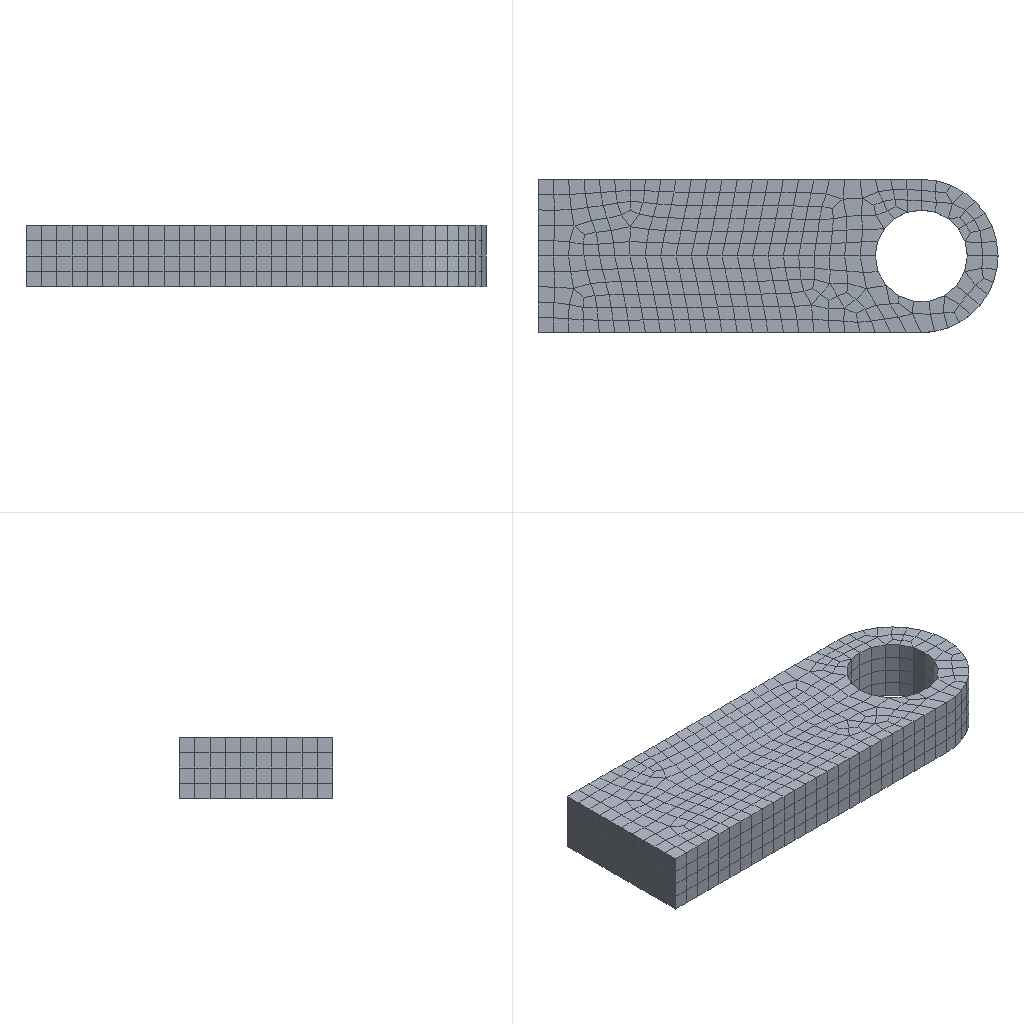Simulation study | abaqus
Set-up summary:
category,name,step,type,value,unit,region
solver,abaqus,,Abaqus/CAE 2024
units,mm-N-s-tonne (MPa),,inferred,E=250000 density=
analysis,Step-1,,static,time_period=1
mesh,nodes,,,1830
mesh,elements,,,1272
element_type,C3D8R,,,1272
material,Material-1,,E,250000
material,Material-1,,nu,0.3
section,Material-1,,solid section,,,_PickedSet5
load,Load-1,Step-1,pressure,50,,_PickedSurf5
bc,BC-1,initial,encastre,[dofs=ENCASTRE],,_PickedSet4
Abaqus input file, long lists of numbers shortened:
*Heading
** Job name: deck Model name: Model-1
** Generated by: Abaqus/CAE 2024
*Preprint, echo=NO, model=NO, history=NO, contact=NO
**
** PARTS
**
*Part, name=Part-1
*Node
      1,          85.,          7.5,          20.
      2,          95.,          7.5,          20.
** (1828 more lines like these left out)
*Element, type=C3D8R
  1,   83,  353,   19,    1,  588, 1179,  708,   95
  2,   22,  354,  373,   23,  691, 1180, 1199,  690
** (1270 more lines like these left out)
*Nset, nset=_PickedSet5, internal, generate
    1,  1830,     1
*Elset, elset=_PickedSet5, internal, generate
    1,  1272,     1
** Section: Section-1
*Solid Section, elset=_PickedSet5, material=Material-1
,
*End Part
**
**
** ASSEMBLY
**
*Assembly, name=Assembly
**
*Instance, name=Part-1-1, part=Part-1
*End Instance
**
*Nset, nset=_PickedSet4, internal, instance=Part-1-1
   4,   5,  12,  13,  16,  17,  51,  52,  53,  54,  84,  85,  86,  87,  88,  89
 132, 133, 134, 135, 199, 200, 201, 202, 211, 212, 213, 225, 226, 227, 228, 513
** (2 more lines like these left out)
*Elset, elset=_PickedSet4, internal, instance=Part-1-1
   16,   35,   36,   37,   78,  177,  196,  197,  198,  239,  338,  357,  358,  359,  400,  499
  518,  519,  520,  561,  660,  682,  683,  684,  735,  817,  839,  840,  841,  892,  974,  996
** (1 more lines like these left out)
*Elset, elset=__PickedSurf5_S6, internal, instance=Part-1-1
  646,  651,  656,  712,  803,  808,  813,  869,  960,  965,  970, 1026, 1117, 1122, 1127, 1183
*Elset, elset=__PickedSurf5_S4, internal, instance=Part-1-1, generate
  650,  1121,   157
*Elset, elset=__PickedSurf5_S3, internal, instance=Part-1-1
  659,  708,  816,  865,  973, 1022, 1130, 1179
*Elset, elset=__PickedSurf5_S5, internal, instance=Part-1-1
  685,  733,  842,  890,  999, 1047, 1156, 1204
*Surface, type=ELEMENT, name=_PickedSurf5, internal
__PickedSurf5_S6, S6
__PickedSurf5_S4, S4
__PickedSurf5_S3, S3
__PickedSurf5_S5, S5
*End Assembly
**
** MATERIALS
**
*Material, name=Material-1
*Elastic
250000., 0.3
**
** BOUNDARY CONDITIONS
**
** Name: BC-1 Type: Symmetry/Antisymmetry/Encastre
*Boundary
_PickedSet4, ENCASTRE
** ----------------------------------------------------------------
**
** STEP: Step-1
**
*Step, name=Step-1, nlgeom=NO
*Static
0.1, 1., 1e-05, 0.1
**
** LOADS
**
** Name: Load-1   Type: Pressure
*Dsload
_PickedSurf5, P, 50.
**
** OUTPUT REQUESTS
**
*Restart, write, frequency=0
**
** FIELD OUTPUT: F-Output-1
**
*Output, field, variable=PRESELECT
**
** HISTORY OUTPUT: H-Output-1
**
*Output, history, variable=PRESELECT
*End Step
Results summary:
result,odb.job_status,,,JOB_STATUS_COMPLETED_SUCCESSFULLY,"consistent, unstated (Abaqus has no unit system)"
result,steps[0].procedure,Step-1,,*STATIC,"consistent, unstated (Abaqus has no unit system)"
result,steps[0].time_period,Step-1,,1,"consistent, unstated (Abaqus has no unit system)"
result,steps[0].n_frames,Step-1,,11,"consistent, unstated (Abaqus has no unit system)"
result,steps[0].last_frame.id,Step-1,,10,"consistent, unstated (Abaqus has no unit system)"
result,steps[0].last_frame.value,Step-1,,1,"consistent, unstated (Abaqus has no unit system)"
result,steps[0].last_frame.description,Step-1,,Increment     10: Step Time =    1.000,"consistent, unstated (Abaqus has no unit system)"
result,steps[0].completed,Step-1,,True,"consistent, unstated (Abaqus has no unit system)"
result,steps[0].max_U_magnitude,Step-1,,0.5733,"consistent, unstated (Abaqus has no unit system)"
result,steps[0].max_S_mises,Step-1,,399.91,"consistent, unstated (Abaqus has no unit system)"
result,steps[0].RF_sum[1],Step-1,,0.0009766,"consistent, unstated (Abaqus has no unit system)"
result,steps[0].RF_sum[2],Step-1,,30000,"consistent, unstated (Abaqus has no unit system)"
result,steps[0].RF_sum[3],Step-1,,-0.0001221,"consistent, unstated (Abaqus has no unit system)"